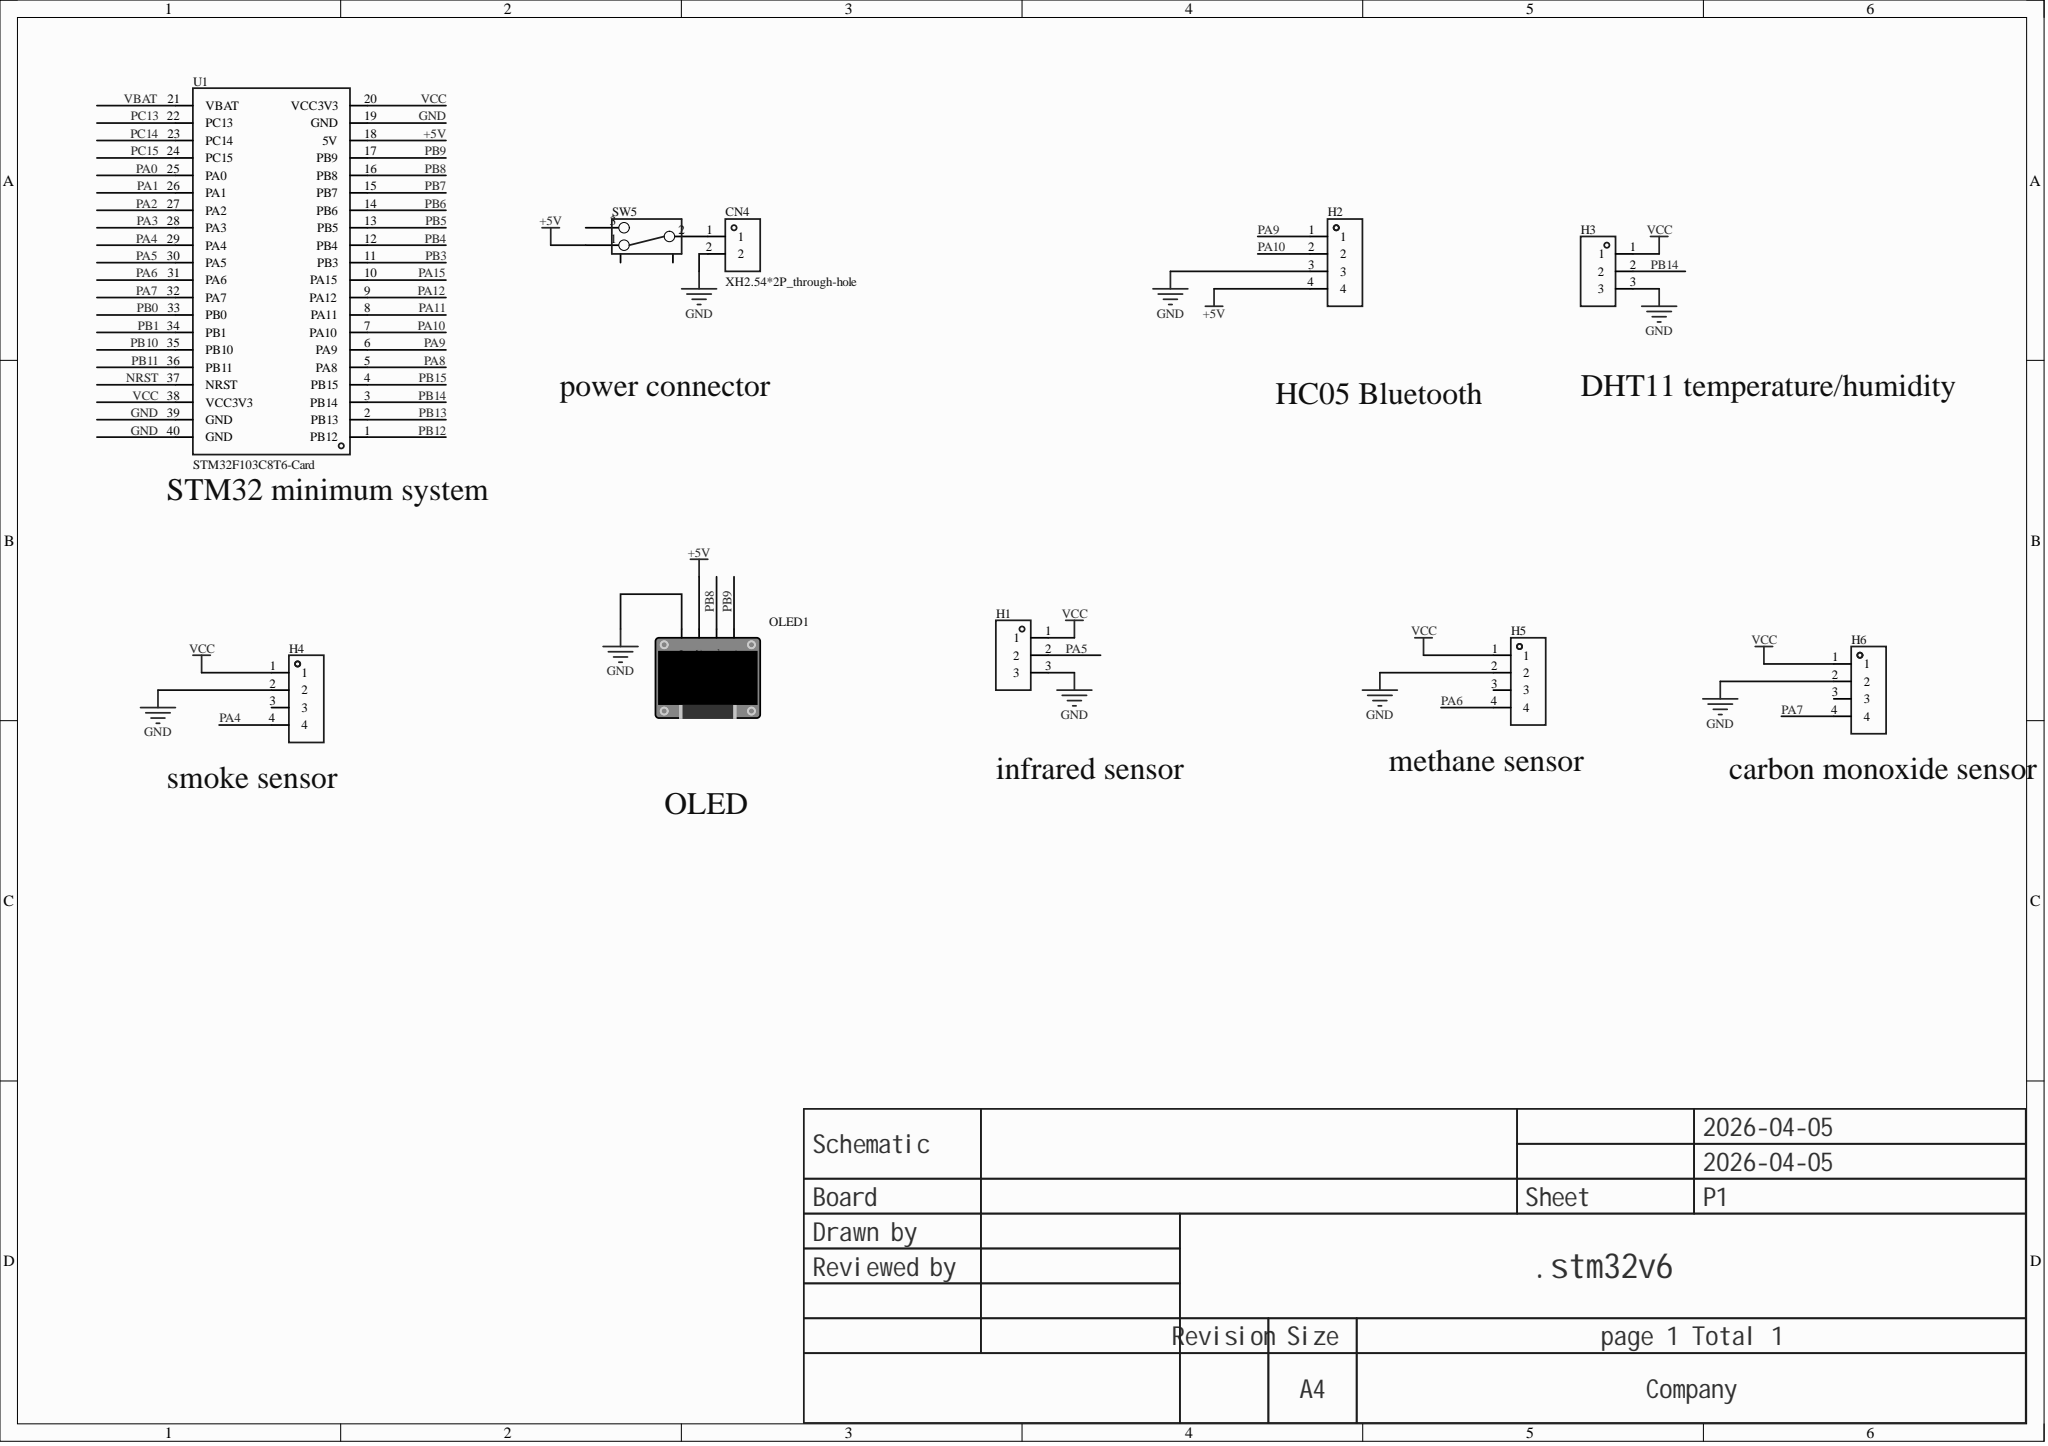Circuit board | Altium Designer | 10 parts | 13 nets
Bill of materials:
Comment,Description,Designator,Footprint,LibRef,Quantity
"XH2.54*2P_through-hole","","CN4","CONN-TH_2P-P2.50-XH2.54-2P","XH2.54*2P_直插","1"
"","","H1, H3","HDR-TH_3P-P2.54-V-F","HDR-F_2.54_1x3P","2"
"","","H2, H4, H5, H6","HDR-TH_4P-P2.54-V-F","HDR-F_2.54_1x4P","4"
"","","OLED1","0.96OLED_4P","0.96OLED模块_4P","1"
"","","SW5","拨动开关","拨动开关_正","1"
"STM32F103C8T6-Card","","U1","CONN-TH_L53.3-W22.9_STM32F103C8T6-CARD","STM32F103C8T6-Card","1"
Netlist (Protel format):
[
CN4
CONN-TH_2P-P2.50-XH2.54-2P
XH2.54*2P_through-hole



]
[
H1
HDR-TH_3P-P2.54-V-F




]
[
H2
HDR-TH_4P-P2.54-V-F




]
[
H3
HDR-TH_3P-P2.54-V-F




]
[
H4
HDR-TH_4P-P2.54-V-F




]
[
H5
HDR-TH_4P-P2.54-V-F




]
[
H6
HDR-TH_4P-P2.54-V-F




]
[
OLED1
0.96OLED_4P




]
[
SW5
拨动开关




]
[
U1
CONN-TH_L53.3-W22.9_STM32F103C8T6-CARD
STM32F103C8T6-Card



]
(
VCC
H1-1
H3-1
H4-1
H5-1
H6-1
U1-20
U1-38
)
(
PB14
H3-2
U1-3
)
(
PB9
OLED1-4
U1-17
)
(
PB8
OLED1-3
U1-16
)
(
PA10
H2-2
U1-7
)
(
PA9
H2-1
U1-6
)
(
PA7
H6-4
U1-32
)
(
PA6
H5-4
U1-31
)
(
PA5
H1-2
U1-30
)
(
PA4
H4-4
U1-29
)
(
NetCN4_1
CN4-1
SW5-2
)
(
GND
CN4-2
H1-3
H2-3
H3-3
H4-2
H5-2
H6-2
OLED1-1
U1-19
U1-39
U1-40
)
(
+5V
H2-4
OLED1-2
SW5-1
U1-18
)